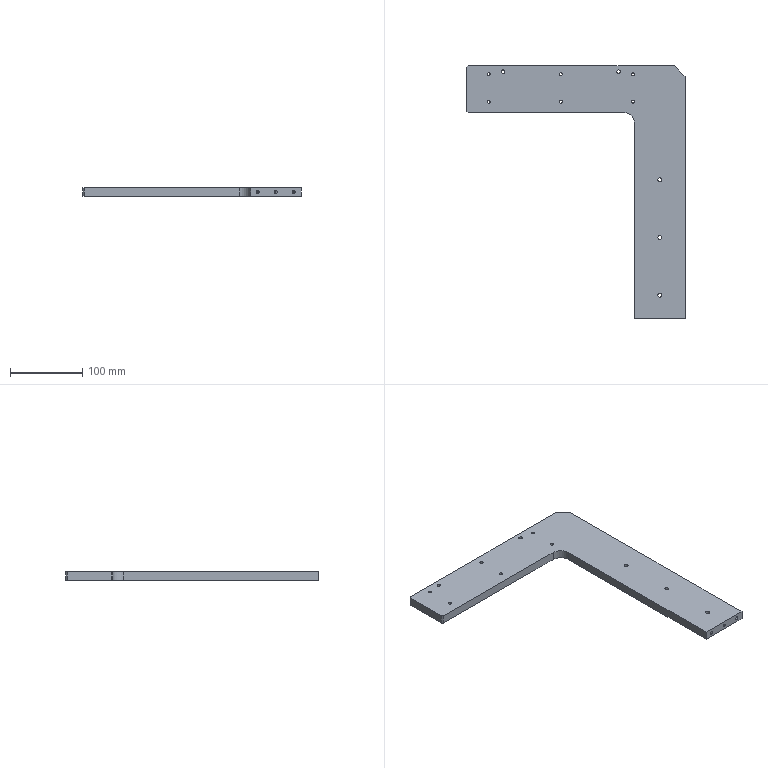Part | STEP file | PN_0060 Mount electronic clip mounting plate 7 | 1 solid | 55 faces | box 302 x 350 x 12 mm | volume 470281 mm3 | cylinder 35 | plane 14 | cone 6 | commonest cylinder face diameters 4.2 x18 5.5 x6 10 x6 5 x4 30 x1